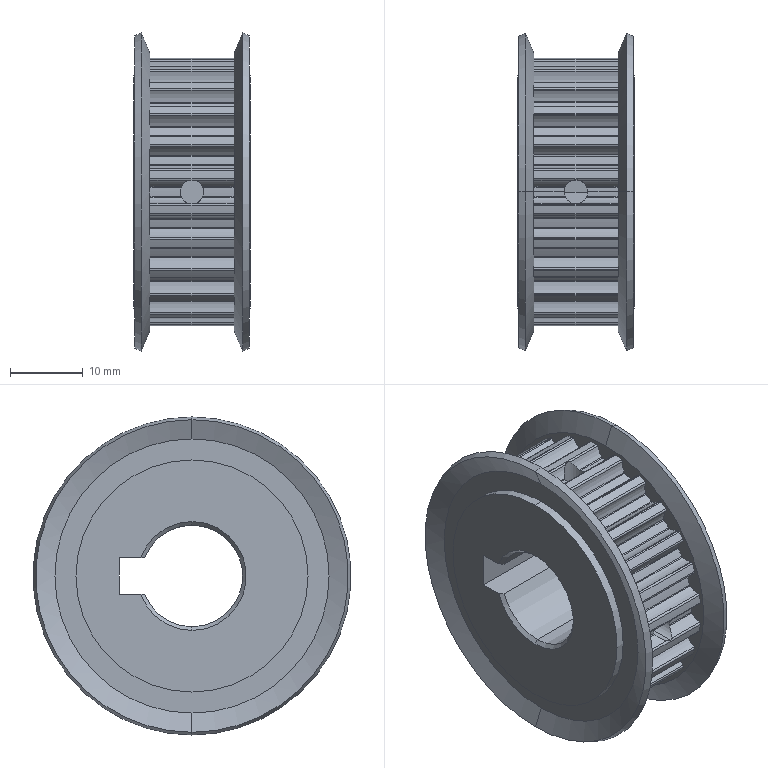Part | SolidWorks | features ICE 3, HoleWzd 2, Chamfer 1, RevCut 1, Revolution 1 | 1 solid | 266 faces | box 16 x 43.859 x 43.859 mm | volume 13285 mm3 | cylinder 239 | cone 18 | plane 9 | commonest cylinder face diameters 0.4 x60 0.5 x60 6.64 x56 33.44 x28 37.06 x24 3.3 x4